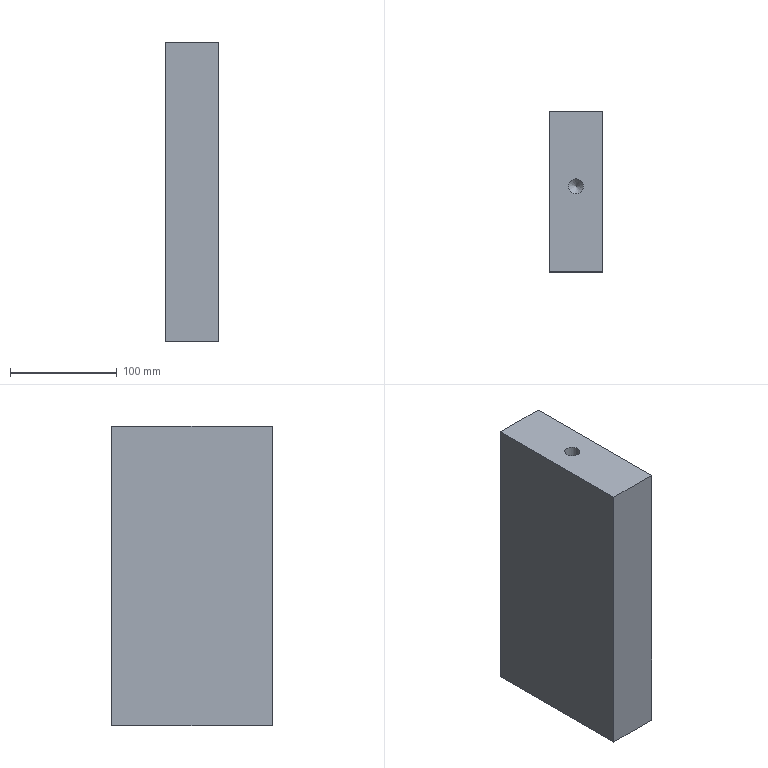Part | NX | features 29 2 | 1 solid | 12 faces | box 50 x 150 x 280.5 mm | volume 2085341 mm3 | plane 6 | cylinder 3 | cone 3 | commonest cylinder face diameters 14.1 x3
STEP:
#1=CARTESIAN_POINT('',(1447.05,-647.5,-493.5));
#2=VERTEX_POINT('',#1);
#3=CARTESIAN_POINT('',(1440.,-647.5,-493.5));
#4=DIRECTION('',(0.,0.,1.));
#5=DIRECTION('',(1.,0.,0.));
#6=AXIS2_PLACEMENT_3D('',#3,#4,#5);
#7=CIRCLE('',#6,7.05);
#8=EDGE_CURVE('',#2,#2,#7,.T.);
#9=ORIENTED_EDGE('',*,*,#8,.T.);
#10=EDGE_LOOP('',(#9));
#11=FACE_BOUND('',#10,.T.);
#12=CARTESIAN_POINT('',(1465.,-522.5,-493.5));
#13=VERTEX_POINT('',#12);
#14=CARTESIAN_POINT('',(1465.,-672.5,-493.5));
#15=VERTEX_POINT('',#14);
#16=CARTESIAN_POINT('',(1465.,-193.,-493.5));
#17=DIRECTION('',(0.,-1.,0.));
#18=VECTOR('',#17,1000.);
#19=LINE('',#16,#18);
#20=EDGE_CURVE('',#13,#15,#19,.T.);
#21=ORIENTED_EDGE('',*,*,#20,.T.);
#22=CARTESIAN_POINT('',(1415.,-672.5,-493.5));
#23=VERTEX_POINT('',#22);
#24=CARTESIAN_POINT('',(972.5,-672.5,-493.5));
#25=DIRECTION('',(1.,0.,0.));
#26=VECTOR('',#25,1000.);
#27=LINE('',#24,#26);
#28=EDGE_CURVE('',#23,#15,#27,.T.);
#29=ORIENTED_EDGE('',*,*,#28,.F.);
#30=CARTESIAN_POINT('',(1415.,-522.5,-493.5));
#31=VERTEX_POINT('',#30);
#32=CARTESIAN_POINT('',(1415.,-193.,-493.5));
#33=DIRECTION('',(0.,1.,0.));
#34=VECTOR('',#33,1000.);
#35=LINE('',#32,#34);
#36=EDGE_CURVE('',#23,#31,#35,.T.);
#37=ORIENTED_EDGE('',*,*,#36,.T.);
#38=CARTESIAN_POINT('',(985.,-522.5,-493.5));
#39=DIRECTION('',(-1.,0.,0.));
#40=VECTOR('',#39,1000.);
#41=LINE('',#38,#40);
#42=EDGE_CURVE('',#13,#31,#41,.T.);
#43=ORIENTED_EDGE('',*,*,#42,.F.);
#44=EDGE_LOOP('',(#21,#29,#37,#43));
#45=FACE_BOUND('',#44,.T.);
#46=CARTESIAN_POINT('',(1447.05,-550.5,-493.5));
#47=VERTEX_POINT('',#46);
#48=CARTESIAN_POINT('',(1440.,-550.5,-493.5));
#49=DIRECTION('',(0.,0.,1.));
#50=DIRECTION('',(1.,0.,0.));
#51=AXIS2_PLACEMENT_3D('',#48,#49,#50);
#52=CIRCLE('',#51,7.05);
#53=EDGE_CURVE('',#47,#47,#52,.T.);
#54=ORIENTED_EDGE('',*,*,#53,.T.);
#55=EDGE_LOOP('',(#54));
#56=FACE_BOUND('',#55,.T.);
#57=CARTESIAN_POINT('',(985.,0.,-493.5));
#58=DIRECTION('',(0.,0.,-1.));
#59=DIRECTION('',(1.,0.,0.));
#60=AXIS2_PLACEMENT_3D('',#57,#58,#59);
#61=PLANE('',#60);
#62=ADVANCED_FACE('',(#11,#45,#56),#61,.T.);
#63=CARTESIAN_POINT('',(1415.,-522.5,-213.));
#64=VERTEX_POINT('',#63);
#65=CARTESIAN_POINT('',(1415.,-672.5,-213.));
#66=VERTEX_POINT('',#65);
#67=CARTESIAN_POINT('',(1415.,-193.,-213.));
#68=DIRECTION('',(0.,-1.,0.));
#69=VECTOR('',#68,1000.);
#70=LINE('',#67,#69);
#71=EDGE_CURVE('',#64,#66,#70,.T.);
#72=ORIENTED_EDGE('',*,*,#71,.T.);
#73=CARTESIAN_POINT('',(1465.,-672.5,-213.));
#74=VERTEX_POINT('',#73);
#75=CARTESIAN_POINT('',(972.5,-672.5,-213.));
#76=DIRECTION('',(-1.,0.,0.));
#77=VECTOR('',#76,1000.);
#78=LINE('',#75,#77);
#79=EDGE_CURVE('',#74,#66,#78,.T.);
#80=ORIENTED_EDGE('',*,*,#79,.F.);
#81=CARTESIAN_POINT('',(1465.,-522.5,-213.));
#82=VERTEX_POINT('',#81);
#83=CARTESIAN_POINT('',(1465.,-193.,-213.));
#84=DIRECTION('',(0.,1.,0.));
#85=VECTOR('',#84,1000.);
#86=LINE('',#83,#85);
#87=EDGE_CURVE('',#74,#82,#86,.T.);
#88=ORIENTED_EDGE('',*,*,#87,.T.);
#89=CARTESIAN_POINT('',(985.,-522.5,-213.));
#90=DIRECTION('',(1.,0.,0.));
#91=VECTOR('',#90,1000.);
#92=LINE('',#89,#91);
#93=EDGE_CURVE('',#64,#82,#92,.T.);
#94=ORIENTED_EDGE('',*,*,#93,.F.);
#95=EDGE_LOOP('',(#72,#80,#88,#94));
#96=FACE_BOUND('',#95,.T.);
#97=CARTESIAN_POINT('',(1447.05,-592.5,-213.));
#98=VERTEX_POINT('',#97);
#99=CARTESIAN_POINT('',(1440.,-592.5,-213.));
#100=DIRECTION('',(0.,0.,-1.));
#101=DIRECTION('',(1.,0.,0.));
#102=AXIS2_PLACEMENT_3D('',#99,#100,#101);
#103=CIRCLE('',#102,7.05);
#104=EDGE_CURVE('',#98,#98,#103,.T.);
#105=ORIENTED_EDGE('',*,*,#104,.T.);
#106=EDGE_LOOP('',(#105));
#107=FACE_BOUND('',#106,.T.);
#108=CARTESIAN_POINT('',(985.,0.,-213.));
#109=DIRECTION('',(0.,0.,1.));
#110=DIRECTION('',(-1.,0.,0.));
#111=AXIS2_PLACEMENT_3D('',#108,#109,#110);
#112=PLANE('',#111);
#113=ADVANCED_FACE('',(#96,#107),#112,.T.);
#114=ORIENTED_EDGE('',*,*,#93,.T.);
#115=CARTESIAN_POINT('',(1465.,-522.5,-205.5));
#116=DIRECTION('',(0.,0.,-1.));
#117=VECTOR('',#116,1000.);
#118=LINE('',#115,#117);
#119=EDGE_CURVE('',#82,#13,#118,.T.);
#120=ORIENTED_EDGE('',*,*,#119,.T.);
#121=ORIENTED_EDGE('',*,*,#42,.T.);
#122=CARTESIAN_POINT('',(1415.,-522.5,-205.5));
#123=DIRECTION('',(0.,0.,1.));
#124=VECTOR('',#123,1000.);
#125=LINE('',#122,#124);
#126=EDGE_CURVE('',#31,#64,#125,.T.);
#127=ORIENTED_EDGE('',*,*,#126,.T.);
#128=EDGE_LOOP('',(#114,#120,#121,#127));
#129=FACE_BOUND('',#128,.T.);
#130=CARTESIAN_POINT('',(1440.,-522.5,-353.25));
#131=DIRECTION('',(0.,1.,0.));
#132=DIRECTION('',(0.,0.,1.));
#133=AXIS2_PLACEMENT_3D('',#130,#131,#132);
#134=PLANE('',#133);
#135=ADVANCED_FACE('',(#129),#134,.T.);
#136=ORIENTED_EDGE('',*,*,#36,.F.);
#137=CARTESIAN_POINT('',(1415.,-672.5,-205.5));
#138=DIRECTION('',(0.,0.,1.));
#139=VECTOR('',#138,1000.);
#140=LINE('',#137,#139);
#141=EDGE_CURVE('',#23,#66,#140,.T.);
#142=ORIENTED_EDGE('',*,*,#141,.T.);
#143=ORIENTED_EDGE('',*,*,#71,.F.);
#144=ORIENTED_EDGE('',*,*,#126,.F.);
#145=EDGE_LOOP('',(#136,#142,#143,#144));
#146=FACE_BOUND('',#145,.T.);
#147=CARTESIAN_POINT('',(1415.,-193.,-205.5));
#148=DIRECTION('',(-1.,0.,0.));
#149=DIRECTION('',(0.,0.,1.));
#150=AXIS2_PLACEMENT_3D('',#147,#148,#149);
#151=PLANE('',#150);
#152=ADVANCED_FACE('',(#146),#151,.T.);
#153=ORIENTED_EDGE('',*,*,#87,.F.);
#154=CARTESIAN_POINT('',(1465.,-672.5,91.));
#155=DIRECTION('',(0.,0.,1.));
#156=VECTOR('',#155,1000.);
#157=LINE('',#154,#156);
#158=EDGE_CURVE('',#15,#74,#157,.T.);
#159=ORIENTED_EDGE('',*,*,#158,.F.);
#160=ORIENTED_EDGE('',*,*,#20,.F.);
#161=ORIENTED_EDGE('',*,*,#119,.F.);
#162=EDGE_LOOP('',(#153,#159,#160,#161));
#163=FACE_BOUND('',#162,.T.);
#164=CARTESIAN_POINT('',(1465.,-193.,-205.5));
#165=DIRECTION('',(1.,0.,0.));
#166=DIRECTION('',(0.,0.,-1.));
#167=AXIS2_PLACEMENT_3D('',#164,#165,#166);
#168=PLANE('',#167);
#169=ADVANCED_FACE('',(#163),#168,.T.);
#170=ORIENTED_EDGE('',*,*,#28,.T.);
#171=ORIENTED_EDGE('',*,*,#158,.T.);
#172=ORIENTED_EDGE('',*,*,#79,.T.);
#173=ORIENTED_EDGE('',*,*,#141,.F.);
#174=EDGE_LOOP('',(#170,#171,#172,#173));
#175=FACE_BOUND('',#174,.T.);
#176=CARTESIAN_POINT('',(972.5,-672.5,91.));
#177=DIRECTION('',(0.,1.,0.));
#178=DIRECTION('',(-1.,0.,0.));
#179=AXIS2_PLACEMENT_3D('',#176,#177,#178);
#180=PLANE('',#179);
#181=ADVANCED_FACE('',(#175),#180,.F.);
#182=CARTESIAN_POINT('',(1432.95,-592.5,-249.95));
#183=VERTEX_POINT('',#182);
#184=CARTESIAN_POINT('',(1440.,-592.5,-249.95));
#185=DIRECTION('',(0.,0.,-1.));
#186=DIRECTION('',(-1.,0.,0.));
#187=AXIS2_PLACEMENT_3D('',#184,#185,#186);
#188=CIRCLE('',#187,7.05);
#189=EDGE_CURVE('',#183,#183,#188,.T.);
#190=ORIENTED_EDGE('',*,*,#189,.T.);
#191=EDGE_LOOP('',(#190));
#192=FACE_BOUND('',#191,.T.);
#193=ORIENTED_EDGE('',*,*,#104,.F.);
#194=EDGE_LOOP('',(#193));
#195=FACE_BOUND('',#194,.T.);
#196=CARTESIAN_POINT('',(1440.,-592.5,-213.));
#197=DIRECTION('',(0.,0.,-1.));
#198=DIRECTION('',(-1.,0.,0.));
#199=AXIS2_PLACEMENT_3D('',#196,#197,#198);
#200=CYLINDRICAL_SURFACE('',#199,7.05);
#201=ADVANCED_FACE('',(#192,#195),#200,.F.);
#202=CARTESIAN_POINT('',(1440.,-592.5,-257.));
#203=VERTEX_POINT('',#202);
#204=VERTEX_LOOP('',#203);
#205=FACE_BOUND('',#204,.T.);
#206=ORIENTED_EDGE('',*,*,#189,.F.);
#207=EDGE_LOOP('',(#206));
#208=FACE_BOUND('',#207,.T.);
#209=CARTESIAN_POINT('',(1440.,-592.5,-249.95));
#210=DIRECTION('',(0.,0.,1.));
#211=DIRECTION('',(-1.,0.,0.));
#212=AXIS2_PLACEMENT_3D('',#209,#210,#211);
#213=CONICAL_SURFACE('',#212,7.05,0.7854);
#214=ADVANCED_FACE('',(#205,#208),#213,.F.);
#215=CARTESIAN_POINT('',(1447.05,-647.5,-456.55));
#216=VERTEX_POINT('',#215);
#217=CARTESIAN_POINT('',(1440.,-647.5,-456.55));
#218=DIRECTION('',(0.,0.,1.));
#219=DIRECTION('',(1.,0.,0.));
#220=AXIS2_PLACEMENT_3D('',#217,#218,#219);
#221=CIRCLE('',#220,7.05);
#222=EDGE_CURVE('',#216,#216,#221,.T.);
#223=ORIENTED_EDGE('',*,*,#222,.T.);
#224=EDGE_LOOP('',(#223));
#225=FACE_BOUND('',#224,.T.);
#226=ORIENTED_EDGE('',*,*,#8,.F.);
#227=EDGE_LOOP('',(#226));
#228=FACE_BOUND('',#227,.T.);
#229=CARTESIAN_POINT('',(1440.,-647.5,-493.5));
#230=DIRECTION('',(0.,0.,1.));
#231=DIRECTION('',(-1.,0.,0.));
#232=AXIS2_PLACEMENT_3D('',#229,#230,#231);
#233=CYLINDRICAL_SURFACE('',#232,7.05);
#234=ADVANCED_FACE('',(#225,#228),#233,.F.);
#235=CARTESIAN_POINT('',(1440.,-647.5,-449.5));
#236=VERTEX_POINT('',#235);
#237=VERTEX_LOOP('',#236);
#238=FACE_BOUND('',#237,.T.);
#239=ORIENTED_EDGE('',*,*,#222,.F.);
#240=EDGE_LOOP('',(#239));
#241=FACE_BOUND('',#240,.T.);
#242=CARTESIAN_POINT('',(1440.,-647.5,-456.55));
#243=DIRECTION('',(0.,0.,-1.));
#244=DIRECTION('',(1.,0.,0.));
#245=AXIS2_PLACEMENT_3D('',#242,#243,#244);
#246=CONICAL_SURFACE('',#245,7.05,0.7854);
#247=ADVANCED_FACE('',(#238,#241),#246,.F.);
#248=CARTESIAN_POINT('',(1447.05,-550.5,-456.55));
#249=VERTEX_POINT('',#248);
#250=CARTESIAN_POINT('',(1440.,-550.5,-456.55));
#251=DIRECTION('',(0.,0.,1.));
#252=DIRECTION('',(1.,0.,0.));
#253=AXIS2_PLACEMENT_3D('',#250,#251,#252);
#254=CIRCLE('',#253,7.05);
#255=EDGE_CURVE('',#249,#249,#254,.T.);
#256=ORIENTED_EDGE('',*,*,#255,.T.);
#257=EDGE_LOOP('',(#256));
#258=FACE_BOUND('',#257,.T.);
#259=ORIENTED_EDGE('',*,*,#53,.F.);
#260=EDGE_LOOP('',(#259));
#261=FACE_BOUND('',#260,.T.);
#262=CARTESIAN_POINT('',(1440.,-550.5,-493.5));
#263=DIRECTION('',(0.,0.,1.));
#264=DIRECTION('',(-1.,0.,0.));
#265=AXIS2_PLACEMENT_3D('',#262,#263,#264);
#266=CYLINDRICAL_SURFACE('',#265,7.05);
#267=ADVANCED_FACE('',(#258,#261),#266,.F.);
#268=CARTESIAN_POINT('',(1440.,-550.5,-449.5));
#269=VERTEX_POINT('',#268);
#270=VERTEX_LOOP('',#269);
#271=FACE_BOUND('',#270,.T.);
#272=ORIENTED_EDGE('',*,*,#255,.F.);
#273=EDGE_LOOP('',(#272));
#274=FACE_BOUND('',#273,.T.);
#275=CARTESIAN_POINT('',(1440.,-550.5,-456.55));
#276=DIRECTION('',(0.,0.,-1.));
#277=DIRECTION('',(1.,0.,0.));
#278=AXIS2_PLACEMENT_3D('',#275,#276,#277);
#279=CONICAL_SURFACE('',#278,7.05,0.7854);
#280=ADVANCED_FACE('',(#271,#274),#279,.F.);
#281=CLOSED_SHELL('',(#62,#113,#135,#152,#169,#181,#201,#214,#234,#247,#267,#280));
#282=MANIFOLD_SOLID_BREP('',#281);
#283=(LENGTH_UNIT()NAMED_UNIT(*)SI_UNIT(.MILLI.,.METRE.));
#284=UNCERTAINTY_MEASURE_WITH_UNIT(LENGTH_MEASURE(0.00001),#283,'','');
#285=(NAMED_UNIT(*)PLANE_ANGLE_UNIT()SI_UNIT($,.RADIAN.));
#286=(NAMED_UNIT(*)SI_UNIT($,.STERADIAN.)SOLID_ANGLE_UNIT());
#287=(GEOMETRIC_REPRESENTATION_CONTEXT(3)GLOBAL_UNCERTAINTY_ASSIGNED_CONTEXT((#284))GLOBAL_UNIT_ASSIGNED_CONTEXT((#283,#285,#286))REPRESENTATION_CONTEXT('',''));
#288=ADVANCED_BREP_SHAPE_REPRESENTATION('',(#282),#287);